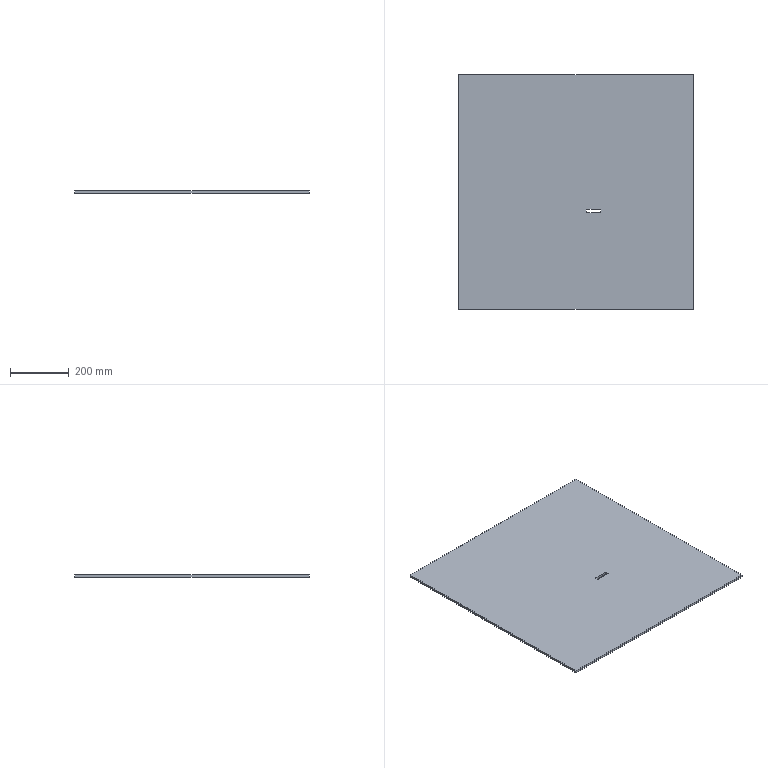Part | STEP file | Bass plate | 1 solid | 14 faces | box 800 x 800 x 8 mm | volume 5115227 mm3 | plane 10 | cylinder 4 | commonest cylinder face diameters 4 x4
STEP:
#1=CARTESIAN_POINT('',(400.,-400.,0.));
#2=VERTEX_POINT('',#1);
#3=CARTESIAN_POINT('',(400.,400.,0.));
#4=VERTEX_POINT('',#3);
#5=CARTESIAN_POINT('',(400.,-400.,0.));
#6=DIRECTION('',(0.,1.,0.));
#7=VECTOR('',#6,1000.);
#8=LINE('',#5,#7);
#9=EDGE_CURVE('',#2,#4,#8,.T.);
#10=ORIENTED_EDGE('',*,*,#9,.T.);
#11=CARTESIAN_POINT('',(400.,400.,8.));
#12=VERTEX_POINT('',#11);
#13=CARTESIAN_POINT('',(400.,400.,8.));
#14=DIRECTION('',(0.,0.,-1.));
#15=VECTOR('',#14,1000.);
#16=LINE('',#13,#15);
#17=EDGE_CURVE('',#12,#4,#16,.T.);
#18=ORIENTED_EDGE('',*,*,#17,.F.);
#19=CARTESIAN_POINT('',(400.,-400.,8.));
#20=VERTEX_POINT('',#19);
#21=CARTESIAN_POINT('',(400.,-400.,8.));
#22=DIRECTION('',(0.,1.,0.));
#23=VECTOR('',#22,1000.);
#24=LINE('',#21,#23);
#25=EDGE_CURVE('',#20,#12,#24,.T.);
#26=ORIENTED_EDGE('',*,*,#25,.F.);
#27=CARTESIAN_POINT('',(400.,-400.,8.));
#28=DIRECTION('',(0.,0.,-1.));
#29=VECTOR('',#28,1000.);
#30=LINE('',#27,#29);
#31=EDGE_CURVE('',#20,#2,#30,.T.);
#32=ORIENTED_EDGE('',*,*,#31,.T.);
#33=EDGE_LOOP('',(#10,#18,#26,#32));
#34=FACE_OUTER_BOUND('',#33,.T.);
#35=CARTESIAN_POINT('',(400.,-400.,8.));
#36=DIRECTION('',(-1.,0.,0.));
#37=DIRECTION('',(0.,0.,1.));
#38=AXIS2_PLACEMENT_3D('',#35,#36,#37);
#39=PLANE('',#38);
#40=ADVANCED_FACE('',(#34),#39,.F.);
#41=CARTESIAN_POINT('',(-400.,400.,0.));
#42=VERTEX_POINT('',#41);
#43=CARTESIAN_POINT('',(-400.,400.,0.));
#44=DIRECTION('',(-1.,0.,0.));
#45=VECTOR('',#44,1000.);
#46=LINE('',#43,#45);
#47=EDGE_CURVE('',#4,#42,#46,.T.);
#48=ORIENTED_EDGE('',*,*,#47,.T.);
#49=CARTESIAN_POINT('',(-400.,400.,8.));
#50=VERTEX_POINT('',#49);
#51=CARTESIAN_POINT('',(-400.,400.,8.));
#52=DIRECTION('',(0.,0.,-1.));
#53=VECTOR('',#52,1000.);
#54=LINE('',#51,#53);
#55=EDGE_CURVE('',#50,#42,#54,.T.);
#56=ORIENTED_EDGE('',*,*,#55,.F.);
#57=CARTESIAN_POINT('',(-400.,400.,8.));
#58=DIRECTION('',(-1.,0.,0.));
#59=VECTOR('',#58,1000.);
#60=LINE('',#57,#59);
#61=EDGE_CURVE('',#12,#50,#60,.T.);
#62=ORIENTED_EDGE('',*,*,#61,.F.);
#63=ORIENTED_EDGE('',*,*,#17,.T.);
#64=EDGE_LOOP('',(#48,#56,#62,#63));
#65=FACE_OUTER_BOUND('',#64,.T.);
#66=CARTESIAN_POINT('',(-400.,400.,8.));
#67=DIRECTION('',(0.,-1.,0.));
#68=DIRECTION('',(0.,0.,-1.));
#69=AXIS2_PLACEMENT_3D('',#66,#67,#68);
#70=PLANE('',#69);
#71=ADVANCED_FACE('',(#65),#70,.F.);
#72=CARTESIAN_POINT('',(-400.,-400.,0.));
#73=VERTEX_POINT('',#72);
#74=CARTESIAN_POINT('',(-400.,-400.,0.));
#75=DIRECTION('',(0.,-1.,0.));
#76=VECTOR('',#75,1000.);
#77=LINE('',#74,#76);
#78=EDGE_CURVE('',#42,#73,#77,.T.);
#79=ORIENTED_EDGE('',*,*,#78,.T.);
#80=CARTESIAN_POINT('',(-400.,-400.,8.));
#81=VERTEX_POINT('',#80);
#82=CARTESIAN_POINT('',(-400.,-400.,8.));
#83=DIRECTION('',(0.,0.,-1.));
#84=VECTOR('',#83,1000.);
#85=LINE('',#82,#84);
#86=EDGE_CURVE('',#81,#73,#85,.T.);
#87=ORIENTED_EDGE('',*,*,#86,.F.);
#88=CARTESIAN_POINT('',(-400.,-400.,8.));
#89=DIRECTION('',(0.,-1.,0.));
#90=VECTOR('',#89,1000.);
#91=LINE('',#88,#90);
#92=EDGE_CURVE('',#50,#81,#91,.T.);
#93=ORIENTED_EDGE('',*,*,#92,.F.);
#94=ORIENTED_EDGE('',*,*,#55,.T.);
#95=EDGE_LOOP('',(#79,#87,#93,#94));
#96=FACE_OUTER_BOUND('',#95,.T.);
#97=CARTESIAN_POINT('',(-400.,-400.,8.));
#98=DIRECTION('',(1.,0.,0.));
#99=DIRECTION('',(0.,0.,-1.));
#100=AXIS2_PLACEMENT_3D('',#97,#98,#99);
#101=PLANE('',#100);
#102=ADVANCED_FACE('',(#96),#101,.F.);
#103=CARTESIAN_POINT('',(-400.,-400.,0.));
#104=DIRECTION('',(1.,0.,0.));
#105=VECTOR('',#104,1000.);
#106=LINE('',#103,#105);
#107=EDGE_CURVE('',#73,#2,#106,.T.);
#108=ORIENTED_EDGE('',*,*,#107,.T.);
#109=ORIENTED_EDGE('',*,*,#31,.F.);
#110=CARTESIAN_POINT('',(-400.,-400.,8.));
#111=DIRECTION('',(1.,0.,0.));
#112=VECTOR('',#111,1000.);
#113=LINE('',#110,#112);
#114=EDGE_CURVE('',#81,#20,#113,.T.);
#115=ORIENTED_EDGE('',*,*,#114,.F.);
#116=ORIENTED_EDGE('',*,*,#86,.T.);
#117=EDGE_LOOP('',(#108,#109,#115,#116));
#118=FACE_OUTER_BOUND('',#117,.T.);
#119=CARTESIAN_POINT('',(-400.,-400.,8.));
#120=DIRECTION('',(0.,1.,0.));
#121=DIRECTION('',(0.,0.,1.));
#122=AXIS2_PLACEMENT_3D('',#119,#120,#121);
#123=PLANE('',#122);
#124=ADVANCED_FACE('',(#118),#123,.F.);
#125=CARTESIAN_POINT('',(37.,-71.,8.));
#126=VERTEX_POINT('',#125);
#127=CARTESIAN_POINT('',(83.,-71.,8.));
#128=VERTEX_POINT('',#127);
#129=CARTESIAN_POINT('',(83.,-71.,8.));
#130=DIRECTION('',(1.,0.,0.));
#131=VECTOR('',#130,1000.);
#132=LINE('',#129,#131);
#133=EDGE_CURVE('',#126,#128,#132,.T.);
#134=ORIENTED_EDGE('',*,*,#133,.F.);
#135=CARTESIAN_POINT('',(35.,-69.,8.));
#136=VERTEX_POINT('',#135);
#137=CARTESIAN_POINT('',(37.,-69.,8.));
#138=DIRECTION('',(0.,0.,1.));
#139=DIRECTION('',(-1.,0.,0.));
#140=AXIS2_PLACEMENT_3D('',#137,#138,#139);
#141=CIRCLE('',#140,2.);
#142=EDGE_CURVE('',#136,#126,#141,.T.);
#143=ORIENTED_EDGE('',*,*,#142,.F.);
#144=CARTESIAN_POINT('',(35.,-61.,8.));
#145=VERTEX_POINT('',#144);
#146=CARTESIAN_POINT('',(35.,-69.,8.));
#147=DIRECTION('',(0.,-1.,0.));
#148=VECTOR('',#147,1000.);
#149=LINE('',#146,#148);
#150=EDGE_CURVE('',#145,#136,#149,.T.);
#151=ORIENTED_EDGE('',*,*,#150,.F.);
#152=CARTESIAN_POINT('',(37.,-59.,8.));
#153=VERTEX_POINT('',#152);
#154=CARTESIAN_POINT('',(37.,-61.,8.));
#155=DIRECTION('',(0.,0.,1.));
#156=DIRECTION('',(-1.,0.,0.));
#157=AXIS2_PLACEMENT_3D('',#154,#155,#156);
#158=CIRCLE('',#157,2.);
#159=EDGE_CURVE('',#153,#145,#158,.T.);
#160=ORIENTED_EDGE('',*,*,#159,.F.);
#161=CARTESIAN_POINT('',(83.,-59.,8.));
#162=VERTEX_POINT('',#161);
#163=CARTESIAN_POINT('',(83.,-59.,8.));
#164=DIRECTION('',(-1.,0.,0.));
#165=VECTOR('',#164,1000.);
#166=LINE('',#163,#165);
#167=EDGE_CURVE('',#162,#153,#166,.T.);
#168=ORIENTED_EDGE('',*,*,#167,.F.);
#169=CARTESIAN_POINT('',(85.,-61.,8.));
#170=VERTEX_POINT('',#169);
#171=CARTESIAN_POINT('',(83.,-61.,8.));
#172=DIRECTION('',(0.,0.,1.));
#173=DIRECTION('',(-1.,0.,0.));
#174=AXIS2_PLACEMENT_3D('',#171,#172,#173);
#175=CIRCLE('',#174,2.);
#176=EDGE_CURVE('',#170,#162,#175,.T.);
#177=ORIENTED_EDGE('',*,*,#176,.F.);
#178=CARTESIAN_POINT('',(85.,-69.,8.));
#179=VERTEX_POINT('',#178);
#180=CARTESIAN_POINT('',(85.,-69.,8.));
#181=DIRECTION('',(0.,1.,0.));
#182=VECTOR('',#181,1000.);
#183=LINE('',#180,#182);
#184=EDGE_CURVE('',#179,#170,#183,.T.);
#185=ORIENTED_EDGE('',*,*,#184,.F.);
#186=CARTESIAN_POINT('',(83.,-69.,8.));
#187=DIRECTION('',(0.,0.,1.));
#188=DIRECTION('',(-1.,0.,0.));
#189=AXIS2_PLACEMENT_3D('',#186,#187,#188);
#190=CIRCLE('',#189,2.);
#191=EDGE_CURVE('',#128,#179,#190,.T.);
#192=ORIENTED_EDGE('',*,*,#191,.F.);
#193=EDGE_LOOP('',(#134,#143,#151,#160,#168,#177,#185,#192));
#194=FACE_BOUND('',#193,.T.);
#195=ORIENTED_EDGE('',*,*,#25,.T.);
#196=ORIENTED_EDGE('',*,*,#61,.T.);
#197=ORIENTED_EDGE('',*,*,#92,.T.);
#198=ORIENTED_EDGE('',*,*,#114,.T.);
#199=EDGE_LOOP('',(#195,#196,#197,#198));
#200=FACE_OUTER_BOUND('',#199,.T.);
#201=CARTESIAN_POINT('',(0.,0.,8.));
#202=DIRECTION('',(0.,0.,-1.));
#203=DIRECTION('',(-1.,0.,0.));
#204=AXIS2_PLACEMENT_3D('',#201,#202,#203);
#205=PLANE('',#204);
#206=ADVANCED_FACE('',(#194,#200),#205,.F.);
#207=CARTESIAN_POINT('',(37.,-71.,0.));
#208=VERTEX_POINT('',#207);
#209=CARTESIAN_POINT('',(35.,-69.,0.));
#210=VERTEX_POINT('',#209);
#211=CARTESIAN_POINT('',(37.,-69.,0.));
#212=DIRECTION('',(0.,0.,-1.));
#213=DIRECTION('',(-1.,0.,0.));
#214=AXIS2_PLACEMENT_3D('',#211,#212,#213);
#215=CIRCLE('',#214,2.);
#216=EDGE_CURVE('',#208,#210,#215,.T.);
#217=ORIENTED_EDGE('',*,*,#216,.F.);
#218=CARTESIAN_POINT('',(83.,-71.,0.));
#219=VERTEX_POINT('',#218);
#220=CARTESIAN_POINT('',(83.,-71.,0.));
#221=DIRECTION('',(-1.,0.,0.));
#222=VECTOR('',#221,1000.);
#223=LINE('',#220,#222);
#224=EDGE_CURVE('',#219,#208,#223,.T.);
#225=ORIENTED_EDGE('',*,*,#224,.F.);
#226=CARTESIAN_POINT('',(85.,-69.,0.));
#227=VERTEX_POINT('',#226);
#228=CARTESIAN_POINT('',(83.,-69.,0.));
#229=DIRECTION('',(0.,0.,-1.));
#230=DIRECTION('',(1.,0.,0.));
#231=AXIS2_PLACEMENT_3D('',#228,#229,#230);
#232=CIRCLE('',#231,2.);
#233=EDGE_CURVE('',#227,#219,#232,.T.);
#234=ORIENTED_EDGE('',*,*,#233,.F.);
#235=CARTESIAN_POINT('',(85.,-61.,0.));
#236=VERTEX_POINT('',#235);
#237=CARTESIAN_POINT('',(85.,-69.,0.));
#238=DIRECTION('',(0.,-1.,0.));
#239=VECTOR('',#238,1000.);
#240=LINE('',#237,#239);
#241=EDGE_CURVE('',#236,#227,#240,.T.);
#242=ORIENTED_EDGE('',*,*,#241,.F.);
#243=CARTESIAN_POINT('',(83.,-59.,0.));
#244=VERTEX_POINT('',#243);
#245=CARTESIAN_POINT('',(83.,-61.,0.));
#246=DIRECTION('',(0.,0.,-1.));
#247=DIRECTION('',(1.,0.,0.));
#248=AXIS2_PLACEMENT_3D('',#245,#246,#247);
#249=CIRCLE('',#248,2.);
#250=EDGE_CURVE('',#244,#236,#249,.T.);
#251=ORIENTED_EDGE('',*,*,#250,.F.);
#252=CARTESIAN_POINT('',(37.,-59.,0.));
#253=VERTEX_POINT('',#252);
#254=CARTESIAN_POINT('',(83.,-59.,0.));
#255=DIRECTION('',(1.,0.,0.));
#256=VECTOR('',#255,1000.);
#257=LINE('',#254,#256);
#258=EDGE_CURVE('',#253,#244,#257,.T.);
#259=ORIENTED_EDGE('',*,*,#258,.F.);
#260=CARTESIAN_POINT('',(35.,-61.,0.));
#261=VERTEX_POINT('',#260);
#262=CARTESIAN_POINT('',(37.,-61.,0.));
#263=DIRECTION('',(0.,0.,-1.));
#264=DIRECTION('',(1.,0.,0.));
#265=AXIS2_PLACEMENT_3D('',#262,#263,#264);
#266=CIRCLE('',#265,2.);
#267=EDGE_CURVE('',#261,#253,#266,.T.);
#268=ORIENTED_EDGE('',*,*,#267,.F.);
#269=CARTESIAN_POINT('',(35.,-69.,0.));
#270=DIRECTION('',(0.,1.,0.));
#271=VECTOR('',#270,1000.);
#272=LINE('',#269,#271);
#273=EDGE_CURVE('',#210,#261,#272,.T.);
#274=ORIENTED_EDGE('',*,*,#273,.F.);
#275=EDGE_LOOP('',(#217,#225,#234,#242,#251,#259,#268,#274));
#276=FACE_BOUND('',#275,.T.);
#277=ORIENTED_EDGE('',*,*,#9,.F.);
#278=ORIENTED_EDGE('',*,*,#107,.F.);
#279=ORIENTED_EDGE('',*,*,#78,.F.);
#280=ORIENTED_EDGE('',*,*,#47,.F.);
#281=EDGE_LOOP('',(#277,#278,#279,#280));
#282=FACE_OUTER_BOUND('',#281,.T.);
#283=CARTESIAN_POINT('',(0.,0.,0.));
#284=DIRECTION('',(0.,0.,-1.));
#285=DIRECTION('',(-1.,0.,0.));
#286=AXIS2_PLACEMENT_3D('',#283,#284,#285);
#287=PLANE('',#286);
#288=ADVANCED_FACE('',(#276,#282),#287,.T.);
#289=ORIENTED_EDGE('',*,*,#142,.T.);
#290=CARTESIAN_POINT('',(37.,-71.,8.001));
#291=DIRECTION('',(0.,0.,-1.));
#292=VECTOR('',#291,1000.);
#293=LINE('',#290,#292);
#294=EDGE_CURVE('',#126,#208,#293,.T.);
#295=ORIENTED_EDGE('',*,*,#294,.T.);
#296=ORIENTED_EDGE('',*,*,#216,.T.);
#297=CARTESIAN_POINT('',(35.,-69.,8.001));
#298=DIRECTION('',(0.,0.,-1.));
#299=VECTOR('',#298,1000.);
#300=LINE('',#297,#299);
#301=EDGE_CURVE('',#136,#210,#300,.T.);
#302=ORIENTED_EDGE('',*,*,#301,.F.);
#303=EDGE_LOOP('',(#289,#295,#296,#302));
#304=FACE_OUTER_BOUND('',#303,.T.);
#305=CARTESIAN_POINT('',(37.,-69.,8.001));
#306=DIRECTION('',(0.,0.,-1.));
#307=DIRECTION('',(-1.,0.,0.));
#308=AXIS2_PLACEMENT_3D('',#305,#306,#307);
#309=CYLINDRICAL_SURFACE('',#308,2.);
#310=ADVANCED_FACE('',(#304),#309,.F.);
#311=ORIENTED_EDGE('',*,*,#133,.T.);
#312=CARTESIAN_POINT('',(83.,-71.,8.001));
#313=DIRECTION('',(0.,0.,-1.));
#314=VECTOR('',#313,1000.);
#315=LINE('',#312,#314);
#316=EDGE_CURVE('',#128,#219,#315,.T.);
#317=ORIENTED_EDGE('',*,*,#316,.T.);
#318=ORIENTED_EDGE('',*,*,#224,.T.);
#319=ORIENTED_EDGE('',*,*,#294,.F.);
#320=EDGE_LOOP('',(#311,#317,#318,#319));
#321=FACE_OUTER_BOUND('',#320,.T.);
#322=CARTESIAN_POINT('',(83.,-71.,8.001));
#323=DIRECTION('',(0.,-1.,0.));
#324=DIRECTION('',(0.,0.,-1.));
#325=AXIS2_PLACEMENT_3D('',#322,#323,#324);
#326=PLANE('',#325);
#327=ADVANCED_FACE('',(#321),#326,.F.);
#328=ORIENTED_EDGE('',*,*,#191,.T.);
#329=CARTESIAN_POINT('',(85.,-69.,8.001));
#330=DIRECTION('',(0.,0.,-1.));
#331=VECTOR('',#330,1000.);
#332=LINE('',#329,#331);
#333=EDGE_CURVE('',#179,#227,#332,.T.);
#334=ORIENTED_EDGE('',*,*,#333,.T.);
#335=ORIENTED_EDGE('',*,*,#233,.T.);
#336=ORIENTED_EDGE('',*,*,#316,.F.);
#337=EDGE_LOOP('',(#328,#334,#335,#336));
#338=FACE_OUTER_BOUND('',#337,.T.);
#339=CARTESIAN_POINT('',(83.,-69.,8.001));
#340=DIRECTION('',(0.,0.,-1.));
#341=DIRECTION('',(-1.,0.,0.));
#342=AXIS2_PLACEMENT_3D('',#339,#340,#341);
#343=CYLINDRICAL_SURFACE('',#342,2.);
#344=ADVANCED_FACE('',(#338),#343,.F.);
#345=ORIENTED_EDGE('',*,*,#184,.T.);
#346=CARTESIAN_POINT('',(85.,-61.,8.001));
#347=DIRECTION('',(0.,0.,-1.));
#348=VECTOR('',#347,1000.);
#349=LINE('',#346,#348);
#350=EDGE_CURVE('',#170,#236,#349,.T.);
#351=ORIENTED_EDGE('',*,*,#350,.T.);
#352=ORIENTED_EDGE('',*,*,#241,.T.);
#353=ORIENTED_EDGE('',*,*,#333,.F.);
#354=EDGE_LOOP('',(#345,#351,#352,#353));
#355=FACE_OUTER_BOUND('',#354,.T.);
#356=CARTESIAN_POINT('',(85.,-69.,8.001));
#357=DIRECTION('',(1.,0.,0.));
#358=DIRECTION('',(0.,0.,-1.));
#359=AXIS2_PLACEMENT_3D('',#356,#357,#358);
#360=PLANE('',#359);
#361=ADVANCED_FACE('',(#355),#360,.F.);
#362=ORIENTED_EDGE('',*,*,#176,.T.);
#363=CARTESIAN_POINT('',(83.,-59.,8.001));
#364=DIRECTION('',(0.,0.,-1.));
#365=VECTOR('',#364,1000.);
#366=LINE('',#363,#365);
#367=EDGE_CURVE('',#162,#244,#366,.T.);
#368=ORIENTED_EDGE('',*,*,#367,.T.);
#369=ORIENTED_EDGE('',*,*,#250,.T.);
#370=ORIENTED_EDGE('',*,*,#350,.F.);
#371=EDGE_LOOP('',(#362,#368,#369,#370));
#372=FACE_OUTER_BOUND('',#371,.T.);
#373=CARTESIAN_POINT('',(83.,-61.,8.001));
#374=DIRECTION('',(0.,0.,-1.));
#375=DIRECTION('',(-1.,0.,0.));
#376=AXIS2_PLACEMENT_3D('',#373,#374,#375);
#377=CYLINDRICAL_SURFACE('',#376,2.);
#378=ADVANCED_FACE('',(#372),#377,.F.);
#379=ORIENTED_EDGE('',*,*,#167,.T.);
#380=CARTESIAN_POINT('',(37.,-59.,8.001));
#381=DIRECTION('',(0.,0.,-1.));
#382=VECTOR('',#381,1000.);
#383=LINE('',#380,#382);
#384=EDGE_CURVE('',#153,#253,#383,.T.);
#385=ORIENTED_EDGE('',*,*,#384,.T.);
#386=ORIENTED_EDGE('',*,*,#258,.T.);
#387=ORIENTED_EDGE('',*,*,#367,.F.);
#388=EDGE_LOOP('',(#379,#385,#386,#387));
#389=FACE_OUTER_BOUND('',#388,.T.);
#390=CARTESIAN_POINT('',(83.,-59.,8.001));
#391=DIRECTION('',(0.,1.,0.));
#392=DIRECTION('',(0.,0.,1.));
#393=AXIS2_PLACEMENT_3D('',#390,#391,#392);
#394=PLANE('',#393);
#395=ADVANCED_FACE('',(#389),#394,.F.);
#396=ORIENTED_EDGE('',*,*,#159,.T.);
#397=CARTESIAN_POINT('',(35.,-61.,8.001));
#398=DIRECTION('',(0.,0.,-1.));
#399=VECTOR('',#398,1000.);
#400=LINE('',#397,#399);
#401=EDGE_CURVE('',#145,#261,#400,.T.);
#402=ORIENTED_EDGE('',*,*,#401,.T.);
#403=ORIENTED_EDGE('',*,*,#267,.T.);
#404=ORIENTED_EDGE('',*,*,#384,.F.);
#405=EDGE_LOOP('',(#396,#402,#403,#404));
#406=FACE_OUTER_BOUND('',#405,.T.);
#407=CARTESIAN_POINT('',(37.,-61.,8.001));
#408=DIRECTION('',(0.,0.,-1.));
#409=DIRECTION('',(-1.,0.,0.));
#410=AXIS2_PLACEMENT_3D('',#407,#408,#409);
#411=CYLINDRICAL_SURFACE('',#410,2.);
#412=ADVANCED_FACE('',(#406),#411,.F.);
#413=ORIENTED_EDGE('',*,*,#150,.T.);
#414=ORIENTED_EDGE('',*,*,#301,.T.);
#415=ORIENTED_EDGE('',*,*,#273,.T.);
#416=ORIENTED_EDGE('',*,*,#401,.F.);
#417=EDGE_LOOP('',(#413,#414,#415,#416));
#418=FACE_OUTER_BOUND('',#417,.T.);
#419=CARTESIAN_POINT('',(35.,-69.,8.001));
#420=DIRECTION('',(-1.,0.,0.));
#421=DIRECTION('',(0.,0.,1.));
#422=AXIS2_PLACEMENT_3D('',#419,#420,#421);
#423=PLANE('',#422);
#424=ADVANCED_FACE('',(#418),#423,.F.);
#425=CLOSED_SHELL('',(#40,#71,#102,#124,#206,#288,#310,#327,#344,#361,#378,#395,#412,#424));
#426=MANIFOLD_SOLID_BREP('',#425);
#427=CARTESIAN_POINT('',(0.,0.,0.));
#428=DIRECTION('',(0.,0.,1.));
#429=DIRECTION('',(1.,0.,0.));
#430=AXIS2_PLACEMENT_3D('',#427,#428,#429);
#431=(LENGTH_UNIT()NAMED_UNIT(*)SI_UNIT(.MILLI.,.METRE.));
#432=UNCERTAINTY_MEASURE_WITH_UNIT(LENGTH_MEASURE(0.00001),#431,'','');
#433=(NAMED_UNIT(*)PLANE_ANGLE_UNIT()SI_UNIT($,.RADIAN.));
#434=(NAMED_UNIT(*)SI_UNIT($,.STERADIAN.)SOLID_ANGLE_UNIT());
#435=(GEOMETRIC_REPRESENTATION_CONTEXT(3)GLOBAL_UNCERTAINTY_ASSIGNED_CONTEXT((#432))GLOBAL_UNIT_ASSIGNED_CONTEXT((#431,#433,#434))REPRESENTATION_CONTEXT('',''));
#436=ADVANCED_BREP_SHAPE_REPRESENTATION('',(#426,#430),#435);